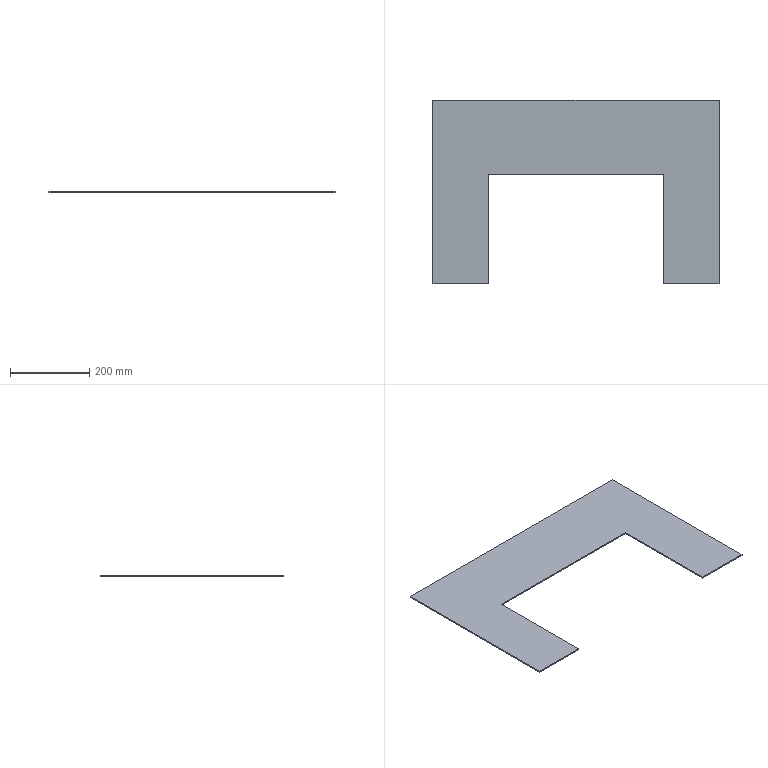Part | STEP file | Guide wheel mechanism revised.sldasm-Part-184 | 1 solid | 10 faces | box 720 x 461.99 x 3 mm | volume 633248 mm3 | plane 10
STEP:
#1=CARTESIAN_POINT('',(-360.,1890.,260.));
#2=VERTEX_POINT('',#1);
#3=CARTESIAN_POINT('',(-360.,1428.01,260.));
#4=VERTEX_POINT('',#3);
#5=CARTESIAN_POINT('',(-360.,1890.,260.));
#6=DIRECTION('',(0.,-1.,0.));
#7=VECTOR('',#6,1000.);
#8=LINE('',#5,#7);
#9=EDGE_CURVE('',#2,#4,#8,.T.);
#10=ORIENTED_EDGE('',*,*,#9,.F.);
#11=CARTESIAN_POINT('',(-360.,1890.,257.));
#12=VERTEX_POINT('',#11);
#13=CARTESIAN_POINT('',(-360.,1890.,257.));
#14=DIRECTION('',(0.,0.,1.));
#15=VECTOR('',#14,1000.);
#16=LINE('',#13,#15);
#17=EDGE_CURVE('',#12,#2,#16,.T.);
#18=ORIENTED_EDGE('',*,*,#17,.F.);
#19=CARTESIAN_POINT('',(-360.,1428.01,257.));
#20=VERTEX_POINT('',#19);
#21=CARTESIAN_POINT('',(-360.,1890.,257.));
#22=DIRECTION('',(0.,-1.,0.));
#23=VECTOR('',#22,1000.);
#24=LINE('',#21,#23);
#25=EDGE_CURVE('',#12,#20,#24,.T.);
#26=ORIENTED_EDGE('',*,*,#25,.T.);
#27=CARTESIAN_POINT('',(-360.,1428.01,257.));
#28=DIRECTION('',(0.,0.,1.));
#29=VECTOR('',#28,1000.);
#30=LINE('',#27,#29);
#31=EDGE_CURVE('',#20,#4,#30,.T.);
#32=ORIENTED_EDGE('',*,*,#31,.T.);
#33=EDGE_LOOP('',(#10,#18,#26,#32));
#34=FACE_OUTER_BOUND('',#33,.T.);
#35=CARTESIAN_POINT('',(-360.,1890.,257.));
#36=DIRECTION('',(-1.,0.,0.));
#37=DIRECTION('',(0.,0.,1.));
#38=AXIS2_PLACEMENT_3D('',#35,#36,#37);
#39=PLANE('',#38);
#40=ADVANCED_FACE('',(#34),#39,.T.);
#41=CARTESIAN_POINT('',(360.,1890.,260.));
#42=VERTEX_POINT('',#41);
#43=CARTESIAN_POINT('',(-360.,1890.,260.));
#44=DIRECTION('',(-1.,0.,0.));
#45=VECTOR('',#44,1000.);
#46=LINE('',#43,#45);
#47=EDGE_CURVE('',#42,#2,#46,.T.);
#48=ORIENTED_EDGE('',*,*,#47,.F.);
#49=CARTESIAN_POINT('',(360.,1890.,257.));
#50=VERTEX_POINT('',#49);
#51=CARTESIAN_POINT('',(360.,1890.,257.));
#52=DIRECTION('',(0.,0.,1.));
#53=VECTOR('',#52,1000.);
#54=LINE('',#51,#53);
#55=EDGE_CURVE('',#50,#42,#54,.T.);
#56=ORIENTED_EDGE('',*,*,#55,.F.);
#57=CARTESIAN_POINT('',(-360.,1890.,257.));
#58=DIRECTION('',(-1.,0.,0.));
#59=VECTOR('',#58,1000.);
#60=LINE('',#57,#59);
#61=EDGE_CURVE('',#50,#12,#60,.T.);
#62=ORIENTED_EDGE('',*,*,#61,.T.);
#63=ORIENTED_EDGE('',*,*,#17,.T.);
#64=EDGE_LOOP('',(#48,#56,#62,#63));
#65=FACE_OUTER_BOUND('',#64,.T.);
#66=CARTESIAN_POINT('',(-360.,1890.,257.));
#67=DIRECTION('',(0.,1.,0.));
#68=DIRECTION('',(0.,0.,1.));
#69=AXIS2_PLACEMENT_3D('',#66,#67,#68);
#70=PLANE('',#69);
#71=ADVANCED_FACE('',(#65),#70,.T.);
#72=CARTESIAN_POINT('',(360.,1428.01,260.));
#73=VERTEX_POINT('',#72);
#74=CARTESIAN_POINT('',(360.,1890.,260.));
#75=DIRECTION('',(0.,1.,0.));
#76=VECTOR('',#75,1000.);
#77=LINE('',#74,#76);
#78=EDGE_CURVE('',#73,#42,#77,.T.);
#79=ORIENTED_EDGE('',*,*,#78,.F.);
#80=CARTESIAN_POINT('',(360.,1428.01,257.));
#81=VERTEX_POINT('',#80);
#82=CARTESIAN_POINT('',(360.,1428.01,257.));
#83=DIRECTION('',(0.,0.,1.));
#84=VECTOR('',#83,1000.);
#85=LINE('',#82,#84);
#86=EDGE_CURVE('',#81,#73,#85,.T.);
#87=ORIENTED_EDGE('',*,*,#86,.F.);
#88=CARTESIAN_POINT('',(360.,1890.,257.));
#89=DIRECTION('',(0.,1.,0.));
#90=VECTOR('',#89,1000.);
#91=LINE('',#88,#90);
#92=EDGE_CURVE('',#81,#50,#91,.T.);
#93=ORIENTED_EDGE('',*,*,#92,.T.);
#94=ORIENTED_EDGE('',*,*,#55,.T.);
#95=EDGE_LOOP('',(#79,#87,#93,#94));
#96=FACE_OUTER_BOUND('',#95,.T.);
#97=CARTESIAN_POINT('',(360.,1890.,257.));
#98=DIRECTION('',(1.,0.,0.));
#99=DIRECTION('',(0.,0.,-1.));
#100=AXIS2_PLACEMENT_3D('',#97,#98,#99);
#101=PLANE('',#100);
#102=ADVANCED_FACE('',(#96),#101,.T.);
#103=CARTESIAN_POINT('',(221.,1428.01,260.));
#104=VERTEX_POINT('',#103);
#105=CARTESIAN_POINT('',(221.,1428.01,260.));
#106=DIRECTION('',(1.,0.,0.));
#107=VECTOR('',#106,1000.);
#108=LINE('',#105,#107);
#109=EDGE_CURVE('',#104,#73,#108,.T.);
#110=ORIENTED_EDGE('',*,*,#109,.F.);
#111=CARTESIAN_POINT('',(221.,1428.01,257.));
#112=VERTEX_POINT('',#111);
#113=CARTESIAN_POINT('',(221.,1428.01,257.));
#114=DIRECTION('',(0.,0.,1.));
#115=VECTOR('',#114,1000.);
#116=LINE('',#113,#115);
#117=EDGE_CURVE('',#112,#104,#116,.T.);
#118=ORIENTED_EDGE('',*,*,#117,.F.);
#119=CARTESIAN_POINT('',(221.,1428.01,257.));
#120=DIRECTION('',(1.,0.,0.));
#121=VECTOR('',#120,1000.);
#122=LINE('',#119,#121);
#123=EDGE_CURVE('',#112,#81,#122,.T.);
#124=ORIENTED_EDGE('',*,*,#123,.T.);
#125=ORIENTED_EDGE('',*,*,#86,.T.);
#126=EDGE_LOOP('',(#110,#118,#124,#125));
#127=FACE_OUTER_BOUND('',#126,.T.);
#128=CARTESIAN_POINT('',(221.,1428.01,257.));
#129=DIRECTION('',(0.,-1.,0.));
#130=DIRECTION('',(1.,0.,0.));
#131=AXIS2_PLACEMENT_3D('',#128,#129,#130);
#132=PLANE('',#131);
#133=ADVANCED_FACE('',(#127),#132,.T.);
#134=CARTESIAN_POINT('',(221.,1703.01,260.));
#135=VERTEX_POINT('',#134);
#136=CARTESIAN_POINT('',(221.,1703.01,260.));
#137=DIRECTION('',(0.,-1.,0.));
#138=VECTOR('',#137,1000.);
#139=LINE('',#136,#138);
#140=EDGE_CURVE('',#135,#104,#139,.T.);
#141=ORIENTED_EDGE('',*,*,#140,.F.);
#142=CARTESIAN_POINT('',(221.,1703.01,257.));
#143=VERTEX_POINT('',#142);
#144=CARTESIAN_POINT('',(221.,1703.01,257.));
#145=DIRECTION('',(0.,0.,1.));
#146=VECTOR('',#145,1000.);
#147=LINE('',#144,#146);
#148=EDGE_CURVE('',#143,#135,#147,.T.);
#149=ORIENTED_EDGE('',*,*,#148,.F.);
#150=CARTESIAN_POINT('',(221.,1703.01,257.));
#151=DIRECTION('',(0.,-1.,0.));
#152=VECTOR('',#151,1000.);
#153=LINE('',#150,#152);
#154=EDGE_CURVE('',#143,#112,#153,.T.);
#155=ORIENTED_EDGE('',*,*,#154,.T.);
#156=ORIENTED_EDGE('',*,*,#117,.T.);
#157=EDGE_LOOP('',(#141,#149,#155,#156));
#158=FACE_OUTER_BOUND('',#157,.T.);
#159=CARTESIAN_POINT('',(221.,1703.01,257.));
#160=DIRECTION('',(-1.,0.,0.));
#161=DIRECTION('',(0.,-1.,0.));
#162=AXIS2_PLACEMENT_3D('',#159,#160,#161);
#163=PLANE('',#162);
#164=ADVANCED_FACE('',(#158),#163,.T.);
#165=CARTESIAN_POINT('',(-221.,1703.01,260.));
#166=VERTEX_POINT('',#165);
#167=CARTESIAN_POINT('',(-221.,1703.01,260.));
#168=DIRECTION('',(1.,0.,0.));
#169=VECTOR('',#168,1000.);
#170=LINE('',#167,#169);
#171=EDGE_CURVE('',#166,#135,#170,.T.);
#172=ORIENTED_EDGE('',*,*,#171,.F.);
#173=CARTESIAN_POINT('',(-221.,1703.01,257.));
#174=VERTEX_POINT('',#173);
#175=CARTESIAN_POINT('',(-221.,1703.01,257.));
#176=DIRECTION('',(0.,0.,1.));
#177=VECTOR('',#176,1000.);
#178=LINE('',#175,#177);
#179=EDGE_CURVE('',#174,#166,#178,.T.);
#180=ORIENTED_EDGE('',*,*,#179,.F.);
#181=CARTESIAN_POINT('',(-221.,1703.01,257.));
#182=DIRECTION('',(1.,0.,0.));
#183=VECTOR('',#182,1000.);
#184=LINE('',#181,#183);
#185=EDGE_CURVE('',#174,#143,#184,.T.);
#186=ORIENTED_EDGE('',*,*,#185,.T.);
#187=ORIENTED_EDGE('',*,*,#148,.T.);
#188=EDGE_LOOP('',(#172,#180,#186,#187));
#189=FACE_OUTER_BOUND('',#188,.T.);
#190=CARTESIAN_POINT('',(-221.,1703.01,257.));
#191=DIRECTION('',(0.,-1.,0.));
#192=DIRECTION('',(0.,0.,-1.));
#193=AXIS2_PLACEMENT_3D('',#190,#191,#192);
#194=PLANE('',#193);
#195=ADVANCED_FACE('',(#189),#194,.T.);
#196=CARTESIAN_POINT('',(-221.,1428.01,260.));
#197=VERTEX_POINT('',#196);
#198=CARTESIAN_POINT('',(-221.,1428.01,260.));
#199=DIRECTION('',(0.,1.,0.));
#200=VECTOR('',#199,1000.);
#201=LINE('',#198,#200);
#202=EDGE_CURVE('',#197,#166,#201,.T.);
#203=ORIENTED_EDGE('',*,*,#202,.F.);
#204=CARTESIAN_POINT('',(-221.,1428.01,257.));
#205=VERTEX_POINT('',#204);
#206=CARTESIAN_POINT('',(-221.,1428.01,257.));
#207=DIRECTION('',(0.,0.,1.));
#208=VECTOR('',#207,1000.);
#209=LINE('',#206,#208);
#210=EDGE_CURVE('',#205,#197,#209,.T.);
#211=ORIENTED_EDGE('',*,*,#210,.F.);
#212=CARTESIAN_POINT('',(-221.,1428.01,257.));
#213=DIRECTION('',(0.,1.,0.));
#214=VECTOR('',#213,1000.);
#215=LINE('',#212,#214);
#216=EDGE_CURVE('',#205,#174,#215,.T.);
#217=ORIENTED_EDGE('',*,*,#216,.T.);
#218=ORIENTED_EDGE('',*,*,#179,.T.);
#219=EDGE_LOOP('',(#203,#211,#217,#218));
#220=FACE_OUTER_BOUND('',#219,.T.);
#221=CARTESIAN_POINT('',(-221.,1428.01,257.));
#222=DIRECTION('',(1.,0.,0.));
#223=DIRECTION('',(0.,1.,0.));
#224=AXIS2_PLACEMENT_3D('',#221,#222,#223);
#225=PLANE('',#224);
#226=ADVANCED_FACE('',(#220),#225,.T.);
#227=CARTESIAN_POINT('',(-360.,1428.01,260.));
#228=DIRECTION('',(1.,0.,0.));
#229=VECTOR('',#228,1000.);
#230=LINE('',#227,#229);
#231=EDGE_CURVE('',#4,#197,#230,.T.);
#232=ORIENTED_EDGE('',*,*,#231,.F.);
#233=ORIENTED_EDGE('',*,*,#31,.F.);
#234=CARTESIAN_POINT('',(-360.,1428.01,257.));
#235=DIRECTION('',(1.,0.,0.));
#236=VECTOR('',#235,1000.);
#237=LINE('',#234,#236);
#238=EDGE_CURVE('',#20,#205,#237,.T.);
#239=ORIENTED_EDGE('',*,*,#238,.T.);
#240=ORIENTED_EDGE('',*,*,#210,.T.);
#241=EDGE_LOOP('',(#232,#233,#239,#240));
#242=FACE_OUTER_BOUND('',#241,.T.);
#243=CARTESIAN_POINT('',(-360.,1428.01,257.));
#244=DIRECTION('',(0.,-1.,0.));
#245=DIRECTION('',(1.,0.,0.));
#246=AXIS2_PLACEMENT_3D('',#243,#244,#245);
#247=PLANE('',#246);
#248=ADVANCED_FACE('',(#242),#247,.T.);
#249=ORIENTED_EDGE('',*,*,#25,.F.);
#250=ORIENTED_EDGE('',*,*,#61,.F.);
#251=ORIENTED_EDGE('',*,*,#92,.F.);
#252=ORIENTED_EDGE('',*,*,#123,.F.);
#253=ORIENTED_EDGE('',*,*,#154,.F.);
#254=ORIENTED_EDGE('',*,*,#185,.F.);
#255=ORIENTED_EDGE('',*,*,#216,.F.);
#256=ORIENTED_EDGE('',*,*,#238,.F.);
#257=EDGE_LOOP('',(#249,#250,#251,#252,#253,#254,#255,#256));
#258=FACE_OUTER_BOUND('',#257,.T.);
#259=CARTESIAN_POINT('',(0.,0.,257.));
#260=DIRECTION('',(0.,0.,1.));
#261=DIRECTION('',(1.,0.,0.));
#262=AXIS2_PLACEMENT_3D('',#259,#260,#261);
#263=PLANE('',#262);
#264=ADVANCED_FACE('',(#258),#263,.F.);
#265=ORIENTED_EDGE('',*,*,#9,.T.);
#266=ORIENTED_EDGE('',*,*,#231,.T.);
#267=ORIENTED_EDGE('',*,*,#202,.T.);
#268=ORIENTED_EDGE('',*,*,#171,.T.);
#269=ORIENTED_EDGE('',*,*,#140,.T.);
#270=ORIENTED_EDGE('',*,*,#109,.T.);
#271=ORIENTED_EDGE('',*,*,#78,.T.);
#272=ORIENTED_EDGE('',*,*,#47,.T.);
#273=EDGE_LOOP('',(#265,#266,#267,#268,#269,#270,#271,#272));
#274=FACE_OUTER_BOUND('',#273,.T.);
#275=CARTESIAN_POINT('',(0.,0.,260.));
#276=DIRECTION('',(0.,0.,1.));
#277=DIRECTION('',(1.,0.,0.));
#278=AXIS2_PLACEMENT_3D('',#275,#276,#277);
#279=PLANE('',#278);
#280=ADVANCED_FACE('',(#274),#279,.T.);
#281=CLOSED_SHELL('',(#40,#71,#102,#133,#164,#195,#226,#248,#264,#280));
#282=MANIFOLD_SOLID_BREP('',#281);
#283=CARTESIAN_POINT('',(0.,0.,0.));
#284=DIRECTION('',(0.,0.,1.));
#285=DIRECTION('',(1.,0.,0.));
#286=AXIS2_PLACEMENT_3D('',#283,#284,#285);
#287=(LENGTH_UNIT()NAMED_UNIT(*)SI_UNIT(.MILLI.,.METRE.));
#288=UNCERTAINTY_MEASURE_WITH_UNIT(LENGTH_MEASURE(0.00001),#287,'','');
#289=(NAMED_UNIT(*)PLANE_ANGLE_UNIT()SI_UNIT($,.RADIAN.));
#290=(NAMED_UNIT(*)SI_UNIT($,.STERADIAN.)SOLID_ANGLE_UNIT());
#291=(GEOMETRIC_REPRESENTATION_CONTEXT(3)GLOBAL_UNCERTAINTY_ASSIGNED_CONTEXT((#288))GLOBAL_UNIT_ASSIGNED_CONTEXT((#287,#289,#290))REPRESENTATION_CONTEXT('',''));
#292=ADVANCED_BREP_SHAPE_REPRESENTATION('',(#282,#286),#291);